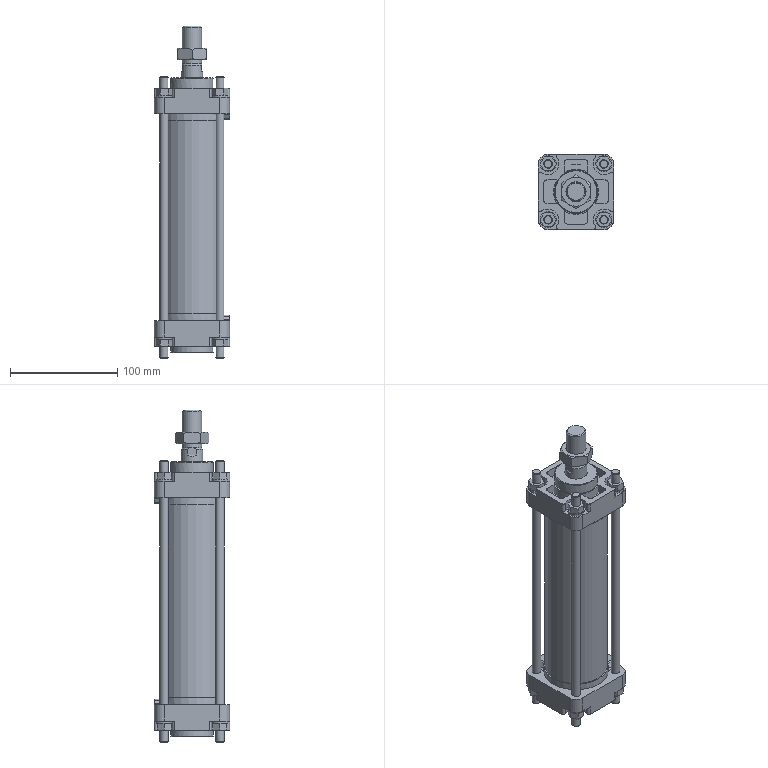Part | NX | features Hydraulic2.1_50 2, Hydraulic2.2_50 2, Hydraulic2.3_M18X1.5 2 | 3 solids | 378 faces | box 70 x 70 x 309 mm | volume 532464 mm3 | plane 234 | cylinder 124 | cone 20 | commonest cylinder face diameters 4 x34 6 x16 5 x12 8 x12 20 x11 18 x10